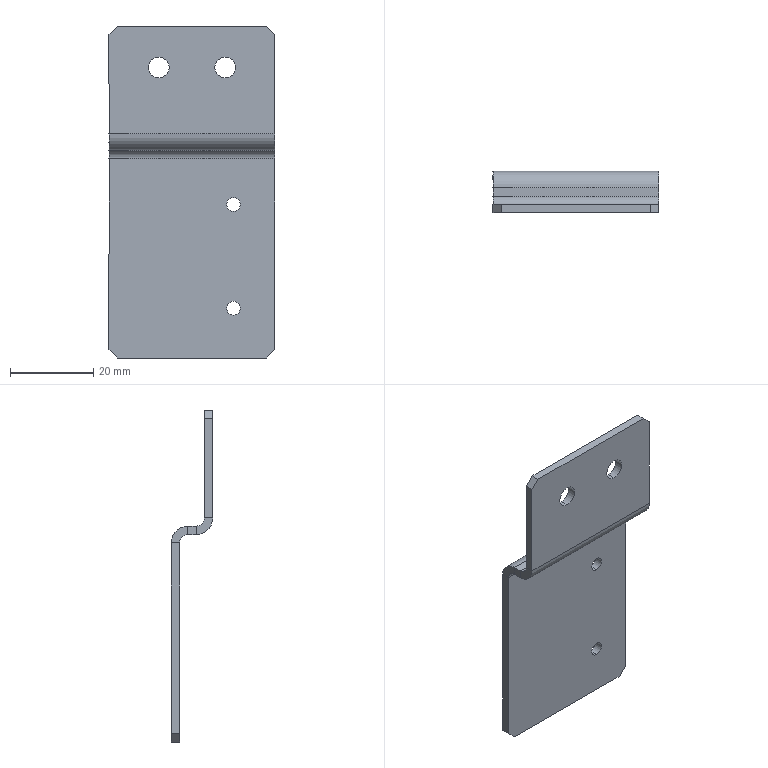Part | STEP file | 227H056252 BKT_Default | 1 solid | 34 faces | box 40 x 10 x 80 mm | volume 6705 mm3 | plane 22 | cylinder 12 | commonest cylinder face diameters 3.3 x4 5 x4 4 x2 8 x2